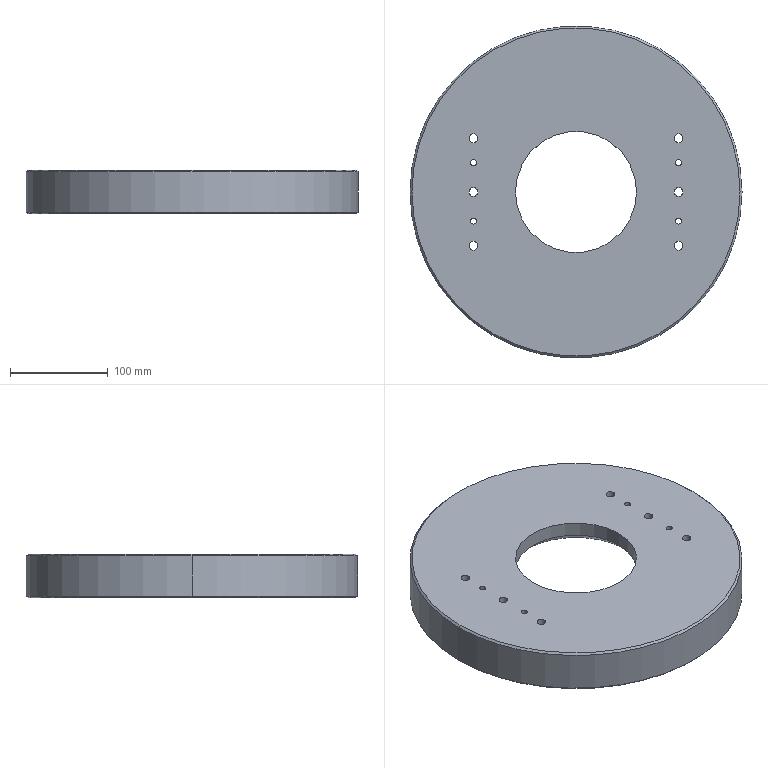NC program | NX | posted with a generic post | part box 340 x 340 x 45 mm
Lines 148 to 925 of 19805:
(ZLEVEL_PROFILE , TOOL : D10)
N294 T10 M6
N296 G54
N298 G17 G0 G90 X-168.713 Y-46.868 S7000 M3
N300 G43 Z75. H10
N302 Z46.5
N304 G94 G1 X-170.667 Y-39.285 Z46.09 F1000.
N306 X-172.476 Y-30.373 Z45.613
N308 X-173.82 Y-21.379 Z45.136
N310 X-174.696 Y-12.327 Z44.66
N312 X-175.1 Y-3.241 Z44.183
N314 Y0. Z44.013
N316 Y0.024 F3000.
N318 G2 X0.024 Y175.1 R175.1
N320 X-175.1 Y0. R-175.1
N322 G1 Y0.387 Z44.007
N324 X-175.098 Y0.774 Z44.
N326 X-175.096 Y1.161 Z43.993
N328 X-175.093 Y1.549 Z43.986
N330 X-175.089 Y1.936 Z43.98
N332 X-175.085 Y2.323 Z43.973
N334 X-175.079 Y2.71 Z43.966
N336 X-175.073 Y3.097 Z43.959
N338 X-175.065 Y3.484 Z43.953
N340 X-175.057 Y3.871 Z43.946
N342 X-175.048 Y4.258 Z43.939
N344 X-175.038 Y4.645 Z43.932
N346 X-175.028 Y5.032 Z43.925
N348 X-175.016 Y5.419 Z43.919
N350 X-175.004 Y5.806 Z43.912
N352 X-174.99 Y6.193 Z43.905
N354 X-174.976 Y6.58 Z43.898
N356 X-174.961 Y6.967 Z43.892
N358 X-174.946 Y7.354 Z43.885
N360 X-174.929 Y7.741 Z43.878
N362 X-174.911 Y8.128 Z43.871
N364 X-174.893 Y8.514 Z43.865
N366 X-174.874 Y8.901 Z43.858
N368 X-174.854 Y9.288 Z43.851
N370 X-174.833 Y9.674 Z43.844
N372 X-174.811 Y10.061 Z43.838
N374 X-174.788 Y10.447 Z43.831
N376 X-174.765 Y10.834 Z43.824
N378 X-174.74 Y11.22 Z43.817
N380 X-174.715 Y11.606 Z43.811
N382 X-174.689 Y11.993 Z43.804
N384 X-174.662 Y12.379 Z43.797
N386 X-174.634 Y12.765 Z43.79
N388 X-174.605 Y13.151 Z43.784
N390 X-174.576 Y13.537 Z43.777
N392 X-174.546 Y13.923 Z43.77
N394 X-174.514 Y14.309 Z43.763
N396 X-174.482 Y14.695 Z43.757
N398 X-174.449 Y15.081 Z43.75
N400 X-174.416 Y15.466 Z43.743
N402 X-174.381 Y15.852 Z43.736
N404 X-174.345 Y16.238 Z43.729
N406 X-174.309 Y16.623 Z43.723
N408 X-174.272 Y17.008 Z43.716
N410 X-174.234 Y17.394 Z43.709
N412 X-174.195 Y17.779 Z43.702
N414 X-174.155 Y18.164 Z43.696
N416 X-174.115 Y18.549 Z43.689
N418 X-174.073 Y18.934 Z43.682
N420 X-174.031 Y19.319 Z43.675
N422 X-173.988 Y19.704 Z43.669
N424 X-173.944 Y20.088 Z43.662
N426 X-173.899 Y20.473 Z43.655
N428 X-173.853 Y20.857 Z43.648
N430 X-173.807 Y21.242 Z43.642
N432 X-173.759 Y21.626 Z43.635
N434 X-173.711 Y22.01 Z43.628
N436 X-173.662 Y22.394 Z43.621
N438 X-173.612 Y22.778 Z43.615
N440 X-173.561 Y23.162 Z43.608
N442 X-173.51 Y23.546 Z43.601
N444 X-173.457 Y23.929 Z43.594
N446 X-173.404 Y24.313 Z43.588
N448 X-173.35 Y24.696 Z43.581
N450 X-173.295 Y25.079 Z43.574
N452 X-173.239 Y25.462 Z43.567
N454 X-173.182 Y25.845 Z43.561
N456 X-173.125 Y26.228 Z43.554
N458 X-173.066 Y26.611 Z43.547
N460 X-173.007 Y26.993 Z43.54
N462 X-172.947 Y27.376 Z43.534
N464 X-172.886 Y27.758 Z43.527
N466 X-172.824 Y28.14 Z43.52
N468 X-172.761 Y28.523 Z43.513
N470 X-172.698 Y28.904 Z43.506
N472 X-172.634 Y29.286 Z43.5
N474 X-172.568 Y29.668 Z43.493
N476 X-172.502 Y30.049 Z43.486
N478 X-172.435 Y30.431 Z43.479
N480 X-172.368 Y30.812 Z43.473
N482 X-172.299 Y31.193 Z43.466
N484 X-172.23 Y31.574 Z43.459
N486 X-172.16 Y31.955 Z43.452
N488 X-172.088 Y32.335 Z43.446
N490 X-172.017 Y32.716 Z43.439
N492 X-171.944 Y33.096 Z43.432
N494 X-171.87 Y33.476 Z43.425
N496 X-171.796 Y33.856 Z43.419
N498 X-171.72 Y34.236 Z43.412
N500 X-171.644 Y34.615 Z43.405
N502 X-171.567 Y34.995 Z43.398
N504 X-171.49 Y35.374 Z43.392
N506 X-171.411 Y35.753 Z43.385
N508 X-171.332 Y36.132 Z43.378
N510 X-171.251 Y36.511 Z43.371
N512 X-171.17 Y36.889 Z43.365
N514 X-171.088 Y37.268 Z43.358
N516 X-171.005 Y37.646 Z43.351
N518 X-170.922 Y38.024 Z43.344
N520 X-170.837 Y38.402 Z43.338
N522 X-170.752 Y38.779 Z43.331
N524 X-170.666 Y39.157 Z43.324
N526 X-170.579 Y39.534 Z43.317
N528 X-170.491 Y39.911 Z43.311
N530 X-170.402 Y40.288 Z43.304
N532 X-170.313 Y40.665 Z43.297
N534 X-170.222 Y41.041 Z43.29
N536 X-170.131 Y41.418 Z43.283
N538 X-170.039 Y41.794 Z43.277
N540 X-169.946 Y42.169 Z43.27
N542 X-169.853 Y42.545 Z43.263
N544 X-169.758 Y42.921 Z43.256
N546 X-169.663 Y43.296 Z43.25
N548 X-169.567 Y43.671 Z43.243
N550 X-169.47 Y44.046 Z43.236
N552 X-169.372 Y44.42 Z43.229
N554 X-169.273 Y44.795 Z43.223
N556 X-169.174 Y45.169 Z43.216
N558 X-169.074 Y45.543 Z43.209
N560 X-168.972 Y45.917 Z43.202
N562 X-168.87 Y46.29 Z43.196
N564 X-168.768 Y46.663 Z43.189
N566 X-168.664 Y47.036 Z43.182
N568 X-168.56 Y47.409 Z43.175
N570 X-168.454 Y47.782 Z43.169
N572 X-168.348 Y48.154 Z43.162
N574 X-168.242 Y48.526 Z43.155
N576 X-168.134 Y48.898 Z43.148
N578 X-168.025 Y49.27 Z43.142
N580 X-167.916 Y49.641 Z43.135
N582 X-167.806 Y50.012 Z43.128
N584 X-167.695 Y50.383 Z43.121
N586 X-167.583 Y50.754 Z43.115
N588 X-167.47 Y51.124 Z43.108
N590 X-167.357 Y51.495 Z43.101
N592 X-167.243 Y51.864 Z43.094
N594 X-167.128 Y52.234 Z43.087
N596 X-167.012 Y52.604 Z43.081
N598 X-166.895 Y52.973 Z43.074
N600 X-166.777 Y53.342 Z43.067
N602 X-166.659 Y53.71 Z43.06
N604 X-166.54 Y54.079 Z43.054
N606 X-166.42 Y54.447 Z43.047
N608 X-166.299 Y54.815 Z43.04
N610 X-166.177 Y55.182 Z43.033
N612 X-166.055 Y55.549 Z43.027
N614 G2 X-175.1 Y0. R-175.1
N616 G1 Y0.387 Z43.02
N618 X-175.098 Y0.774 Z43.013
N620 X-175.096 Y1.161 Z43.006
N622 X-175.093 Y1.549 Z43.
N624 X-175.089 Y1.936 Z42.993
N626 X-175.085 Y2.323 Z42.986
N628 X-175.079 Y2.71 Z42.979
N630 X-175.073 Y3.097 Z42.973
N632 X-175.065 Y3.484 Z42.966
N634 X-175.057 Y3.871 Z42.959
N636 X-175.048 Y4.258 Z42.952
N638 X-175.038 Y4.645 Z42.946
N640 X-175.028 Y5.032 Z42.939
N642 X-175.016 Y5.419 Z42.932
N644 X-175.004 Y5.806 Z42.925
N646 X-174.99 Y6.193 Z42.919
N648 X-174.976 Y6.58 Z42.912
N650 X-174.961 Y6.967 Z42.905
N652 X-174.946 Y7.354 Z42.898
N654 X-174.929 Y7.741 Z42.892
N656 X-174.911 Y8.128 Z42.885
N658 X-174.893 Y8.514 Z42.878
N660 X-174.874 Y8.901 Z42.871
N662 X-174.854 Y9.288 Z42.864
N664 X-174.833 Y9.674 Z42.858
N666 X-174.811 Y10.061 Z42.851
N668 X-174.788 Y10.447 Z42.844
N670 X-174.765 Y10.834 Z42.837
N672 X-174.74 Y11.22 Z42.831
N674 X-174.715 Y11.606 Z42.824
N676 X-174.689 Y11.993 Z42.817
N678 X-174.662 Y12.379 Z42.81
N680 X-174.634 Y12.765 Z42.804
N682 X-174.605 Y13.151 Z42.797
N684 X-174.576 Y13.537 Z42.79
N686 X-174.546 Y13.923 Z42.783
N688 X-174.514 Y14.309 Z42.777
N690 X-174.482 Y14.695 Z42.77
N692 X-174.449 Y15.081 Z42.763
N694 X-174.416 Y15.466 Z42.756
N696 X-174.381 Y15.852 Z42.75
N698 X-174.345 Y16.238 Z42.743
N700 X-174.309 Y16.623 Z42.736
N702 X-174.272 Y17.008 Z42.729
N704 X-174.234 Y17.394 Z42.723
N706 X-174.195 Y17.779 Z42.716
N708 X-174.155 Y18.164 Z42.709
N710 X-174.115 Y18.549 Z42.702
N712 X-174.073 Y18.934 Z42.696
N714 X-174.031 Y19.319 Z42.689
N716 X-173.988 Y19.704 Z42.682
N718 X-173.944 Y20.088 Z42.675
N720 X-173.899 Y20.473 Z42.668
N722 X-173.853 Y20.857 Z42.662
N724 X-173.807 Y21.242 Z42.655
N726 X-173.759 Y21.626 Z42.648
N728 X-173.711 Y22.01 Z42.641
N730 X-173.662 Y22.394 Z42.635
N732 X-173.612 Y22.778 Z42.628
N734 X-173.561 Y23.162 Z42.621
N736 X-173.51 Y23.546 Z42.614
N738 X-173.457 Y23.929 Z42.608
N740 X-173.404 Y24.313 Z42.601
N742 X-173.35 Y24.696 Z42.594
N744 X-173.295 Y25.079 Z42.587
N746 X-173.239 Y25.462 Z42.581
N748 X-173.182 Y25.845 Z42.574
N750 X-173.125 Y26.228 Z42.567
N752 X-173.066 Y26.611 Z42.56
N754 X-173.007 Y26.993 Z42.554
N756 X-172.947 Y27.376 Z42.547
N758 X-172.886 Y27.758 Z42.54
N760 X-172.824 Y28.14 Z42.533
N762 X-172.761 Y28.523 Z42.527
N764 X-172.698 Y28.904 Z42.52
N766 X-172.634 Y29.286 Z42.513
N768 X-172.568 Y29.668 Z42.506
N770 X-172.502 Y30.049 Z42.5
N772 X-172.435 Y30.431 Z42.493
N774 X-172.368 Y30.812 Z42.486
N776 X-172.299 Y31.193 Z42.479
N778 X-172.23 Y31.574 Z42.473
N780 X-172.16 Y31.955 Z42.466
N782 X-172.088 Y32.335 Z42.459
N784 X-172.017 Y32.716 Z42.452
N786 X-171.944 Y33.096 Z42.445
N788 X-171.87 Y33.476 Z42.439
N790 X-171.796 Y33.856 Z42.432
N792 X-171.72 Y34.236 Z42.425
N794 X-171.644 Y34.615 Z42.418
N796 X-171.567 Y34.995 Z42.412
N798 X-171.49 Y35.374 Z42.405
N800 X-171.411 Y35.753 Z42.398
N802 X-171.332 Y36.132 Z42.391
N804 X-171.251 Y36.511 Z42.385
N806 X-171.17 Y36.889 Z42.378
N808 X-171.088 Y37.268 Z42.371
N810 X-171.005 Y37.646 Z42.364
N812 X-170.922 Y38.024 Z42.358
N814 X-170.837 Y38.402 Z42.351
N816 X-170.752 Y38.779 Z42.344
N818 X-170.666 Y39.157 Z42.337
N820 X-170.579 Y39.534 Z42.331
N822 X-170.491 Y39.911 Z42.324
N824 X-170.402 Y40.288 Z42.317
N826 X-170.313 Y40.665 Z42.31
N828 X-170.222 Y41.041 Z42.304
N830 X-170.131 Y41.418 Z42.297
N832 X-170.039 Y41.794 Z42.29
N834 X-169.946 Y42.169 Z42.283
N836 X-169.853 Y42.545 Z42.277
N838 X-169.758 Y42.921 Z42.27
N840 X-169.663 Y43.296 Z42.263
N842 X-169.567 Y43.671 Z42.256
N844 X-169.47 Y44.046 Z42.249
N846 X-169.372 Y44.42 Z42.243
N848 X-169.273 Y44.795 Z42.236
N850 X-169.174 Y45.169 Z42.229
N852 X-169.074 Y45.543 Z42.222
N854 X-168.972 Y45.917 Z42.216
N856 X-168.87 Y46.29 Z42.209
N858 X-168.768 Y46.663 Z42.202
N860 X-168.664 Y47.036 Z42.195
N862 X-168.56 Y47.409 Z42.189
N864 X-168.454 Y47.782 Z42.182
N866 X-168.348 Y48.154 Z42.175
N868 X-168.242 Y48.526 Z42.168
N870 X-168.134 Y48.898 Z42.162
N872 X-168.025 Y49.27 Z42.155
N874 X-167.916 Y49.641 Z42.148
N876 X-167.806 Y50.012 Z42.141
N878 X-167.695 Y50.383 Z42.135
N880 X-167.583 Y50.754 Z42.128
N882 X-167.47 Y51.124 Z42.121
N884 X-167.357 Y51.495 Z42.114
N886 X-167.243 Y51.864 Z42.108
N888 X-167.128 Y52.234 Z42.101
N890 X-167.012 Y52.604 Z42.094
N892 X-166.895 Y52.973 Z42.087
N894 X-166.777 Y53.342 Z42.081
N896 X-166.659 Y53.71 Z42.074
N898 X-166.54 Y54.079 Z42.067
N900 X-166.42 Y54.447 Z42.06
N902 X-166.299 Y54.815 Z42.054
N904 X-166.177 Y55.182 Z42.047
N906 X-166.055 Y55.549 Z42.04
N908 G2 X-175.1 Y0. R-175.1
N910 G1 Y0.387 Z42.033
N912 X-175.098 Y0.774 Z42.026
N914 X-175.096 Y1.161 Z42.02
N916 X-175.093 Y1.549 Z42.013
N918 X-175.089 Y1.936 Z42.006
N920 X-175.085 Y2.323 Z41.999
N922 X-175.079 Y2.71 Z41.993
N924 X-175.073 Y3.097 Z41.986
N926 X-175.065 Y3.484 Z41.979
N928 X-175.057 Y3.871 Z41.972
N930 X-175.048 Y4.258 Z41.966
N932 X-175.038 Y4.645 Z41.959
N934 X-175.028 Y5.032 Z41.952
N936 X-175.016 Y5.419 Z41.945
N938 X-175.004 Y5.806 Z41.939
N940 X-174.99 Y6.193 Z41.932
N942 X-174.976 Y6.58 Z41.925
N944 X-174.961 Y6.967 Z41.918
N946 X-174.946 Y7.354 Z41.912
N948 X-174.929 Y7.741 Z41.905
N950 X-174.911 Y8.128 Z41.898
N952 X-174.893 Y8.514 Z41.891
N954 X-174.874 Y8.901 Z41.885
N956 X-174.854 Y9.288 Z41.878
N958 X-174.833 Y9.674 Z41.871
N960 X-174.811 Y10.061 Z41.864
N962 X-174.788 Y10.447 Z41.858
N964 X-174.765 Y10.834 Z41.851
N966 X-174.74 Y11.22 Z41.844
N968 X-174.715 Y11.606 Z41.837
N970 X-174.689 Y11.993 Z41.831
N972 X-174.662 Y12.379 Z41.824
N974 X-174.634 Y12.765 Z41.817
N976 X-174.605 Y13.151 Z41.81
N978 X-174.576 Y13.537 Z41.803
N980 X-174.546 Y13.923 Z41.797
N982 X-174.514 Y14.309 Z41.79
N984 X-174.482 Y14.695 Z41.783
N986 X-174.449 Y15.081 Z41.776
N988 X-174.416 Y15.466 Z41.77
N990 X-174.381 Y15.852 Z41.763
N992 X-174.345 Y16.238 Z41.756
N994 X-174.309 Y16.623 Z41.749
N996 X-174.272 Y17.008 Z41.743
N998 X-174.234 Y17.394 Z41.736
N1000 X-174.195 Y17.779 Z41.729
N1002 X-174.155 Y18.164 Z41.722
N1004 X-174.115 Y18.549 Z41.716
N1006 X-174.073 Y18.934 Z41.709
N1008 X-174.031 Y19.319 Z41.702
N1010 X-173.988 Y19.704 Z41.695
N1012 X-173.944 Y20.088 Z41.689
N1014 X-173.899 Y20.473 Z41.682
N1016 X-173.853 Y20.857 Z41.675
N1018 X-173.807 Y21.242 Z41.668
N1020 X-173.759 Y21.626 Z41.662
N1022 X-173.711 Y22.01 Z41.655
N1024 X-173.662 Y22.394 Z41.648
N1026 X-173.612 Y22.778 Z41.641
N1028 X-173.561 Y23.162 Z41.635
N1030 X-173.51 Y23.546 Z41.628
N1032 X-173.457 Y23.929 Z41.621
N1034 X-173.404 Y24.313 Z41.614
N1036 X-173.35 Y24.696 Z41.607
N1038 X-173.295 Y25.079 Z41.601
N1040 X-173.239 Y25.462 Z41.594
N1042 X-173.182 Y25.845 Z41.587
N1044 X-173.125 Y26.228 Z41.58
N1046 X-173.066 Y26.611 Z41.574
N1048 X-173.007 Y26.993 Z41.567
N1050 X-172.947 Y27.376 Z41.56
N1052 X-172.886 Y27.758 Z41.553
N1054 X-172.824 Y28.14 Z41.547
N1056 X-172.761 Y28.523 Z41.54
N1058 X-172.698 Y28.904 Z41.533
N1060 X-172.634 Y29.286 Z41.526
N1062 X-172.568 Y29.668 Z41.52
N1064 X-172.502 Y30.049 Z41.513
N1066 X-172.435 Y30.431 Z41.506
N1068 X-172.368 Y30.812 Z41.499
N1070 X-172.299 Y31.193 Z41.493
N1072 X-172.23 Y31.574 Z41.486
N1074 X-172.16 Y31.955 Z41.479
N1076 X-172.088 Y32.335 Z41.472
N1078 X-172.017 Y32.716 Z41.466
N1080 X-171.944 Y33.096 Z41.459
N1082 X-171.87 Y33.476 Z41.452
N1084 X-171.796 Y33.856 Z41.445
N1086 X-171.72 Y34.236 Z41.439
N1088 X-171.644 Y34.615 Z41.432
N1090 X-171.567 Y34.995 Z41.425
N1092 X-171.49 Y35.374 Z41.418
N1094 X-171.411 Y35.753 Z41.412
N1096 X-171.332 Y36.132 Z41.405
N1098 X-171.251 Y36.511 Z41.398
N1100 X-171.17 Y36.889 Z41.391
N1102 X-171.088 Y37.268 Z41.384
N1104 X-171.005 Y37.646 Z41.378
N1106 X-170.922 Y38.024 Z41.371
N1108 X-170.837 Y38.402 Z41.364
N1110 X-170.752 Y38.779 Z41.357
N1112 X-170.666 Y39.157 Z41.351
N1114 X-170.579 Y39.534 Z41.344
N1116 X-170.491 Y39.911 Z41.337
N1118 X-170.402 Y40.288 Z41.33
N1120 X-170.313 Y40.665 Z41.324
N1122 X-170.222 Y41.041 Z41.317
N1124 X-170.131 Y41.418 Z41.31
N1126 X-170.039 Y41.794 Z41.303
N1128 X-169.946 Y42.169 Z41.297
N1130 X-169.853 Y42.545 Z41.29
N1132 X-169.758 Y42.921 Z41.283
N1134 X-169.663 Y43.296 Z41.276
N1136 X-169.567 Y43.671 Z41.27
N1138 X-169.47 Y44.046 Z41.263
N1140 X-169.372 Y44.42 Z41.256
N1142 X-169.273 Y44.795 Z41.249
N1144 X-169.174 Y45.169 Z41.243
N1146 X-169.074 Y45.543 Z41.236
N1148 X-168.972 Y45.917 Z41.229
N1150 X-168.87 Y46.29 Z41.222
N1152 X-168.768 Y46.663 Z41.216
N1154 X-168.664 Y47.036 Z41.209
N1156 X-168.56 Y47.409 Z41.202
N1158 X-168.454 Y47.782 Z41.195
N1160 X-168.348 Y48.154 Z41.188
N1162 X-168.242 Y48.526 Z41.182
N1164 X-168.134 Y48.898 Z41.175
N1166 X-168.025 Y49.27 Z41.168
N1168 X-167.916 Y49.641 Z41.161
N1170 X-167.806 Y50.012 Z41.155
N1172 X-167.695 Y50.383 Z41.148
N1174 X-167.583 Y50.754 Z41.141
N1176 X-167.47 Y51.124 Z41.134
N1178 X-167.357 Y51.495 Z41.128
N1180 X-167.243 Y51.864 Z41.121
N1182 X-167.128 Y52.234 Z41.114
N1184 X-167.012 Y52.604 Z41.107
N1186 X-166.895 Y52.973 Z41.101
N1188 X-166.777 Y53.342 Z41.094
N1190 X-166.659 Y53.71 Z41.087
N1192 X-166.54 Y54.079 Z41.08
N1194 X-166.42 Y54.447 Z41.074
N1196 X-166.299 Y54.815 Z41.067
N1198 X-166.177 Y55.182 Z41.06
N1200 X-166.055 Y55.549 Z41.053
N1202 G2 X-175.1 Y0. R-175.1
N1204 G1 Y0.387 Z41.047
N1206 X-175.098 Y0.774 Z41.04
N1208 X-175.096 Y1.161 Z41.033
N1210 X-175.093 Y1.549 Z41.026
N1212 X-175.089 Y1.936 Z41.02
N1214 X-175.085 Y2.323 Z41.013
N1216 X-175.079 Y2.71 Z41.006
N1218 X-175.073 Y3.097 Z40.999
N1220 X-175.065 Y3.484 Z40.993
N1222 X-175.057 Y3.871 Z40.986
N1224 X-175.048 Y4.258 Z40.979
N1226 X-175.038 Y4.645 Z40.972
N1228 X-175.028 Y5.032 Z40.965
N1230 X-175.016 Y5.419 Z40.959
N1232 X-175.004 Y5.806 Z40.952
N1234 X-174.99 Y6.193 Z40.945
N1236 X-174.976 Y6.58 Z40.938
N1238 X-174.961 Y6.967 Z40.932
N1240 X-174.946 Y7.354 Z40.925
N1242 X-174.929 Y7.741 Z40.918
N1244 X-174.911 Y8.128 Z40.911
N1246 X-174.893 Y8.514 Z40.905
N1248 X-174.874 Y8.901 Z40.898
N1250 X-174.854 Y9.288 Z40.891
N1252 X-174.833 Y9.674 Z40.884
N1254 X-174.811 Y10.061 Z40.878
N1256 X-174.788 Y10.447 Z40.871
N1258 X-174.765 Y10.834 Z40.864
N1260 X-174.74 Y11.22 Z40.857
N1262 X-174.715 Y11.606 Z40.851
N1264 X-174.689 Y11.993 Z40.844
N1266 X-174.662 Y12.379 Z40.837
N1268 X-174.634 Y12.765 Z40.83
N1270 X-174.605 Y13.151 Z40.824
N1272 X-174.576 Y13.537 Z40.817
N1274 X-174.546 Y13.923 Z40.81
N1276 X-174.514 Y14.309 Z40.803
N1278 X-174.482 Y14.695 Z40.797
N1280 X-174.449 Y15.081 Z40.79
N1282 X-174.416 Y15.466 Z40.783
N1284 X-174.381 Y15.852 Z40.776
N1286 X-174.345 Y16.238 Z40.769
N1288 X-174.309 Y16.623 Z40.763
N1290 X-174.272 Y17.008 Z40.756
N1292 X-174.234 Y17.394 Z40.749
N1294 X-174.195 Y17.779 Z40.742
N1296 X-174.155 Y18.164 Z40.736
N1298 X-174.115 Y18.549 Z40.729
N1300 X-174.073 Y18.934 Z40.722
N1302 X-174.031 Y19.319 Z40.715
N1304 X-173.988 Y19.704 Z40.709
N1306 X-173.944 Y20.088 Z40.702
N1308 X-173.899 Y20.473 Z40.695
N1310 X-173.853 Y20.857 Z40.688
N1312 X-173.807 Y21.242 Z40.682
N1314 X-173.759 Y21.626 Z40.675
N1316 X-173.711 Y22.01 Z40.668
N1318 X-173.662 Y22.394 Z40.661
N1320 X-173.612 Y22.778 Z40.655
N1322 X-173.561 Y23.162 Z40.648
N1324 X-173.51 Y23.546 Z40.641
N1326 X-173.457 Y23.929 Z40.634
N1328 X-173.404 Y24.313 Z40.628
N1330 X-173.35 Y24.696 Z40.621
N1332 X-173.295 Y25.079 Z40.614
N1334 X-173.239 Y25.462 Z40.607
N1336 X-173.182 Y25.845 Z40.601
N1338 X-173.125 Y26.228 Z40.594
N1340 X-173.066 Y26.611 Z40.587
N1342 X-173.007 Y26.993 Z40.58
N1344 X-172.947 Y27.376 Z40.574
N1346 X-172.886 Y27.758 Z40.567
N1348 X-172.824 Y28.14 Z40.56
N1350 X-172.761 Y28.523 Z40.553
N1352 X-172.698 Y28.904 Z40.546
N1354 X-172.634 Y29.286 Z40.54
N1356 X-172.568 Y29.668 Z40.533
N1358 X-172.502 Y30.049 Z40.526
N1360 X-172.435 Y30.431 Z40.519
N1362 X-172.368 Y30.812 Z40.513
N1364 X-172.299 Y31.193 Z40.506
N1366 X-172.23 Y31.574 Z40.499
N1368 X-172.16 Y31.955 Z40.492
N1370 X-172.088 Y32.335 Z40.486
N1372 X-172.017 Y32.716 Z40.479
N1374 X-171.944 Y33.096 Z40.472
N1376 X-171.87 Y33.476 Z40.465
N1378 X-171.796 Y33.856 Z40.459
N1380 X-171.72 Y34.236 Z40.452
N1382 X-171.644 Y34.615 Z40.445
N1384 X-171.567 Y34.995 Z40.438
N1386 X-171.49 Y35.374 Z40.432
N1388 X-171.411 Y35.753 Z40.425
N1390 X-171.332 Y36.132 Z40.418
N1392 X-171.251 Y36.511 Z40.411
N1394 X-171.17 Y36.889 Z40.405
N1396 X-171.088 Y37.268 Z40.398
N1398 X-171.005 Y37.646 Z40.391
N1400 X-170.922 Y38.024 Z40.384
N1402 X-170.837 Y38.402 Z40.378
N1404 X-170.752 Y38.779 Z40.371
N1406 X-170.666 Y39.157 Z40.364
N1408 X-170.579 Y39.534 Z40.357
N1410 X-170.491 Y39.911 Z40.351
N1412 X-170.402 Y40.288 Z40.344
N1414 X-170.313 Y40.665 Z40.337
N1416 X-170.222 Y41.041 Z40.33
N1418 X-170.131 Y41.418 Z40.323
N1420 X-170.039 Y41.794 Z40.317
N1422 X-169.946 Y42.169 Z40.31
N1424 X-169.853 Y42.545 Z40.303
N1426 X-169.758 Y42.921 Z40.296
N1428 X-169.663 Y43.296 Z40.29
N1430 X-169.567 Y43.671 Z40.283
N1432 X-169.47 Y44.046 Z40.276
N1434 X-169.372 Y44.42 Z40.269
N1436 X-169.273 Y44.795 Z40.263
N1438 X-169.174 Y45.169 Z40.256
N1440 X-169.074 Y45.543 Z40.249
N1442 X-168.972 Y45.917 Z40.242
N1444 X-168.87 Y46.29 Z40.236
N1446 X-168.768 Y46.663 Z40.229
N1448 X-168.664 Y47.036 Z40.222
N1450 X-168.56 Y47.409 Z40.215
N1452 X-168.454 Y47.782 Z40.209
N1454 X-168.348 Y48.154 Z40.202
N1456 X-168.242 Y48.526 Z40.195
N1458 X-168.134 Y48.898 Z40.188
N1460 X-168.025 Y49.27 Z40.182
N1462 X-167.916 Y49.641 Z40.175
N1464 X-167.806 Y50.012 Z40.168
N1466 X-167.695 Y50.383 Z40.161
N1468 X-167.583 Y50.754 Z40.155
N1470 X-167.47 Y51.124 Z40.148
N1472 X-167.357 Y51.495 Z40.141
N1474 X-167.243 Y51.864 Z40.134
N1476 X-167.128 Y52.234 Z40.127
N1478 X-167.012 Y52.604 Z40.121
N1480 X-166.895 Y52.973 Z40.114
N1482 X-166.777 Y53.342 Z40.107
N1484 X-166.659 Y53.71 Z40.1
N1486 X-166.54 Y54.079 Z40.094
N1488 X-166.42 Y54.447 Z40.087
N1490 X-166.299 Y54.815 Z40.08
N1492 X-166.177 Y55.182 Z40.073
N1494 X-166.055 Y55.549 Z40.067
N1496 G2 X-175.1 Y0. R-175.1
N1498 G1 Y0.387 Z40.06
N1500 X-175.098 Y0.774 Z40.053
N1502 X-175.096 Y1.161 Z40.046
N1504 X-175.093 Y1.549 Z40.04
N1506 X-175.089 Y1.936 Z40.033
N1508 X-175.085 Y2.323 Z40.026
N1510 X-175.079 Y2.71 Z40.019
N1512 X-175.073 Y3.097 Z40.013
N1514 X-175.065 Y3.484 Z40.006
N1516 X-175.057 Y3.871 Z39.999
N1518 X-175.048 Y4.258 Z39.992
N1520 X-175.038 Y4.645 Z39.986
N1522 X-175.028 Y5.032 Z39.979
N1524 X-175.016 Y5.419 Z39.972
N1526 X-175.004 Y5.806 Z39.965
N1528 X-174.99 Y6.193 Z39.959
N1530 X-174.976 Y6.58 Z39.952
N1532 X-174.961 Y6.967 Z39.945
N1534 X-174.946 Y7.354 Z39.938
N1536 X-174.929 Y7.741 Z39.932
N1538 X-174.911 Y8.128 Z39.925
N1540 X-174.893 Y8.514 Z39.918
N1542 X-174.874 Y8.901 Z39.911
N1544 X-174.854 Y9.288 Z39.904
N1546 X-174.833 Y9.674 Z39.898
N1548 X-174.811 Y10.061 Z39.891
N1550 X-174.788 Y10.447 Z39.884
N1552 X-174.765 Y10.834 Z39.877
N1554 X-174.74 Y11.22 Z39.871
N1556 X-174.715 Y11.606 Z39.864
N1558 X-174.689 Y11.993 Z39.857
N1560 X-174.662 Y12.379 Z39.85
N1562 X-174.634 Y12.765 Z39.844
N1564 X-174.605 Y13.151 Z39.837
N1566 X-174.576 Y13.537 Z39.83
N1568 X-174.546 Y13.923 Z39.823
N1570 X-174.514 Y14.309 Z39.817
N1572 X-174.482 Y14.695 Z39.81
N1574 X-174.449 Y15.081 Z39.803
N1576 X-174.416 Y15.466 Z39.796
N1578 X-174.381 Y15.852 Z39.79
N1580 X-174.345 Y16.238 Z39.783
N1582 X-174.309 Y16.623 Z39.776
N1584 X-174.272 Y17.008 Z39.769
N1586 X-174.234 Y17.394 Z39.763
N1588 X-174.195 Y17.779 Z39.756
N1590 X-174.155 Y18.164 Z39.749
N1592 X-174.115 Y18.549 Z39.742
N1594 X-174.073 Y18.934 Z39.736
N1596 X-174.031 Y19.319 Z39.729
N1598 X-173.988 Y19.704 Z39.722
N1600 X-173.944 Y20.088 Z39.715
N1602 X-173.899 Y20.473 Z39.708
N1604 X-173.853 Y20.857 Z39.702
N1606 X-173.807 Y21.242 Z39.695
N1608 X-173.759 Y21.626 Z39.688
N1610 X-173.711 Y22.01 Z39.681
N1612 X-173.662 Y22.394 Z39.675
N1614 X-173.612 Y22.778 Z39.668
N1616 X-173.561 Y23.162 Z39.661
N1618 X-173.51 Y23.546 Z39.654
N1620 X-173.457 Y23.929 Z39.648
N1622 X-173.404 Y24.313 Z39.641
N1624 X-173.35 Y24.696 Z39.634
N1626 X-173.295 Y25.079 Z39.627
N1628 X-173.239 Y25.462 Z39.621
N1630 X-173.182 Y25.845 Z39.614
N1632 X-173.125 Y26.228 Z39.607
N1634 X-173.066 Y26.611 Z39.6
N1636 X-173.007 Y26.993 Z39.594
N1638 X-172.947 Y27.376 Z39.587
N1640 X-172.886 Y27.758 Z39.58
N1642 X-172.824 Y28.14 Z39.573
N1644 X-172.761 Y28.523 Z39.567
N1646 X-172.698 Y28.904 Z39.56
N1648 X-172.634 Y29.286 Z39.553
N1650 X-172.568 Y29.668 Z39.546
N1652 X-172.502 Y30.049 Z39.54
N1654 X-172.435 Y30.431 Z39.533
N1656 X-172.368 Y30.812 Z39.526
N1658 X-172.299 Y31.193 Z39.519
N1660 X-172.23 Y31.574 Z39.513
N1662 X-172.16 Y31.955 Z39.506
N1664 X-172.088 Y32.335 Z39.499
N1666 X-172.017 Y32.716 Z39.492
N1668 X-171.944 Y33.096 Z39.485
N1670 X-171.87 Y33.476 Z39.479
N1672 X-171.796 Y33.856 Z39.472
N1674 X-171.72 Y34.236 Z39.465
N1676 X-171.644 Y34.615 Z39.458
N1678 X-171.567 Y34.995 Z39.452
N1680 X-171.49 Y35.374 Z39.445
N1682 X-171.411 Y35.753 Z39.438
N1684 X-171.332 Y36.132 Z39.431
N1686 X-171.251 Y36.511 Z39.425
N1688 X-171.17 Y36.889 Z39.418
N1690 X-171.088 Y37.268 Z39.411
N1692 X-171.005 Y37.646 Z39.404
N1694 X-170.922 Y38.024 Z39.398
N1696 X-170.837 Y38.402 Z39.391
N1698 X-170.752 Y38.779 Z39.384
N1700 X-170.666 Y39.157 Z39.377
N1702 X-170.579 Y39.534 Z39.371
N1704 X-170.491 Y39.911 Z39.364
N1706 X-170.402 Y40.288 Z39.357
N1708 X-170.313 Y40.665 Z39.35
N1710 X-170.222 Y41.041 Z39.344
N1712 X-170.131 Y41.418 Z39.337
N1714 X-170.039 Y41.794 Z39.33
N1716 X-169.946 Y42.169 Z39.323
N1718 X-169.853 Y42.545 Z39.317
N1720 X-169.758 Y42.921 Z39.31
N1722 X-169.663 Y43.296 Z39.303
N1724 X-169.567 Y43.671 Z39.296
N1726 X-169.47 Y44.046 Z39.289
N1728 X-169.372 Y44.42 Z39.283
N1730 X-169.273 Y44.795 Z39.276
N1732 X-169.174 Y45.169 Z39.269
N1734 X-169.074 Y45.543 Z39.262
N1736 X-168.972 Y45.917 Z39.256
N1738 X-168.87 Y46.29 Z39.249
N1740 X-168.768 Y46.663 Z39.242
N1742 X-168.664 Y47.036 Z39.235
N1744 X-168.56 Y47.409 Z39.229
N1746 X-168.454 Y47.782 Z39.222
N1748 X-168.348 Y48.154 Z39.215
N1750 X-168.242 Y48.526 Z39.208
N1752 X-168.134 Y48.898 Z39.202
N1754 X-168.025 Y49.27 Z39.195
N1756 X-167.916 Y49.641 Z39.188
N1758 X-167.806 Y50.012 Z39.181
N1760 X-167.695 Y50.383 Z39.175
N1762 X-167.583 Y50.754 Z39.168
N1764 X-167.47 Y51.124 Z39.161
N1766 X-167.357 Y51.495 Z39.154
N1768 X-167.243 Y51.864 Z39.148
N1770 X-167.128 Y52.234 Z39.141
N1772 X-167.012 Y52.604 Z39.134
N1774 X-166.895 Y52.973 Z39.127
N1776 X-166.777 Y53.342 Z39.121
N1778 X-166.659 Y53.71 Z39.114
N1780 X-166.54 Y54.079 Z39.107
N1782 X-166.42 Y54.447 Z39.1
N1784 X-166.299 Y54.815 Z39.094
N1786 X-166.177 Y55.182 Z39.087
N1788 X-166.055 Y55.549 Z39.08
N1790 G2 X-175.1 Y0. R-175.1
N1792 G1 Y0.387 Z39.073
N1794 X-175.098 Y0.774 Z39.066
N1796 X-175.096 Y1.161 Z39.06
N1798 X-175.093 Y1.549 Z39.053
N1800 X-175.089 Y1.936 Z39.046
N1802 X-175.085 Y2.323 Z39.039
N1804 X-175.079 Y2.71 Z39.033
N1806 X-175.073 Y3.097 Z39.026
N1808 X-175.065 Y3.484 Z39.019
N1810 X-175.057 Y3.871 Z39.012
N1812 X-175.048 Y4.258 Z39.006
N1814 X-175.038 Y4.645 Z38.999
N1816 X-175.028 Y5.032 Z38.992
N1818 X-175.016 Y5.419 Z38.985
N1820 X-175.004 Y5.806 Z38.979
N1822 X-174.99 Y6.193 Z38.972
N1824 X-174.976 Y6.58 Z38.965
N1826 X-174.961 Y6.967 Z38.958
N1828 X-174.946 Y7.354 Z38.952
N1830 X-174.929 Y7.741 Z38.945
N1832 X-174.911 Y8.128 Z38.938
N1834 X-174.893 Y8.514 Z38.931
N1836 X-174.874 Y8.901 Z38.925
N1838 X-174.854 Y9.288 Z38.918
N1840 X-174.833 Y9.674 Z38.911
N1842 X-174.811 Y10.061 Z38.904